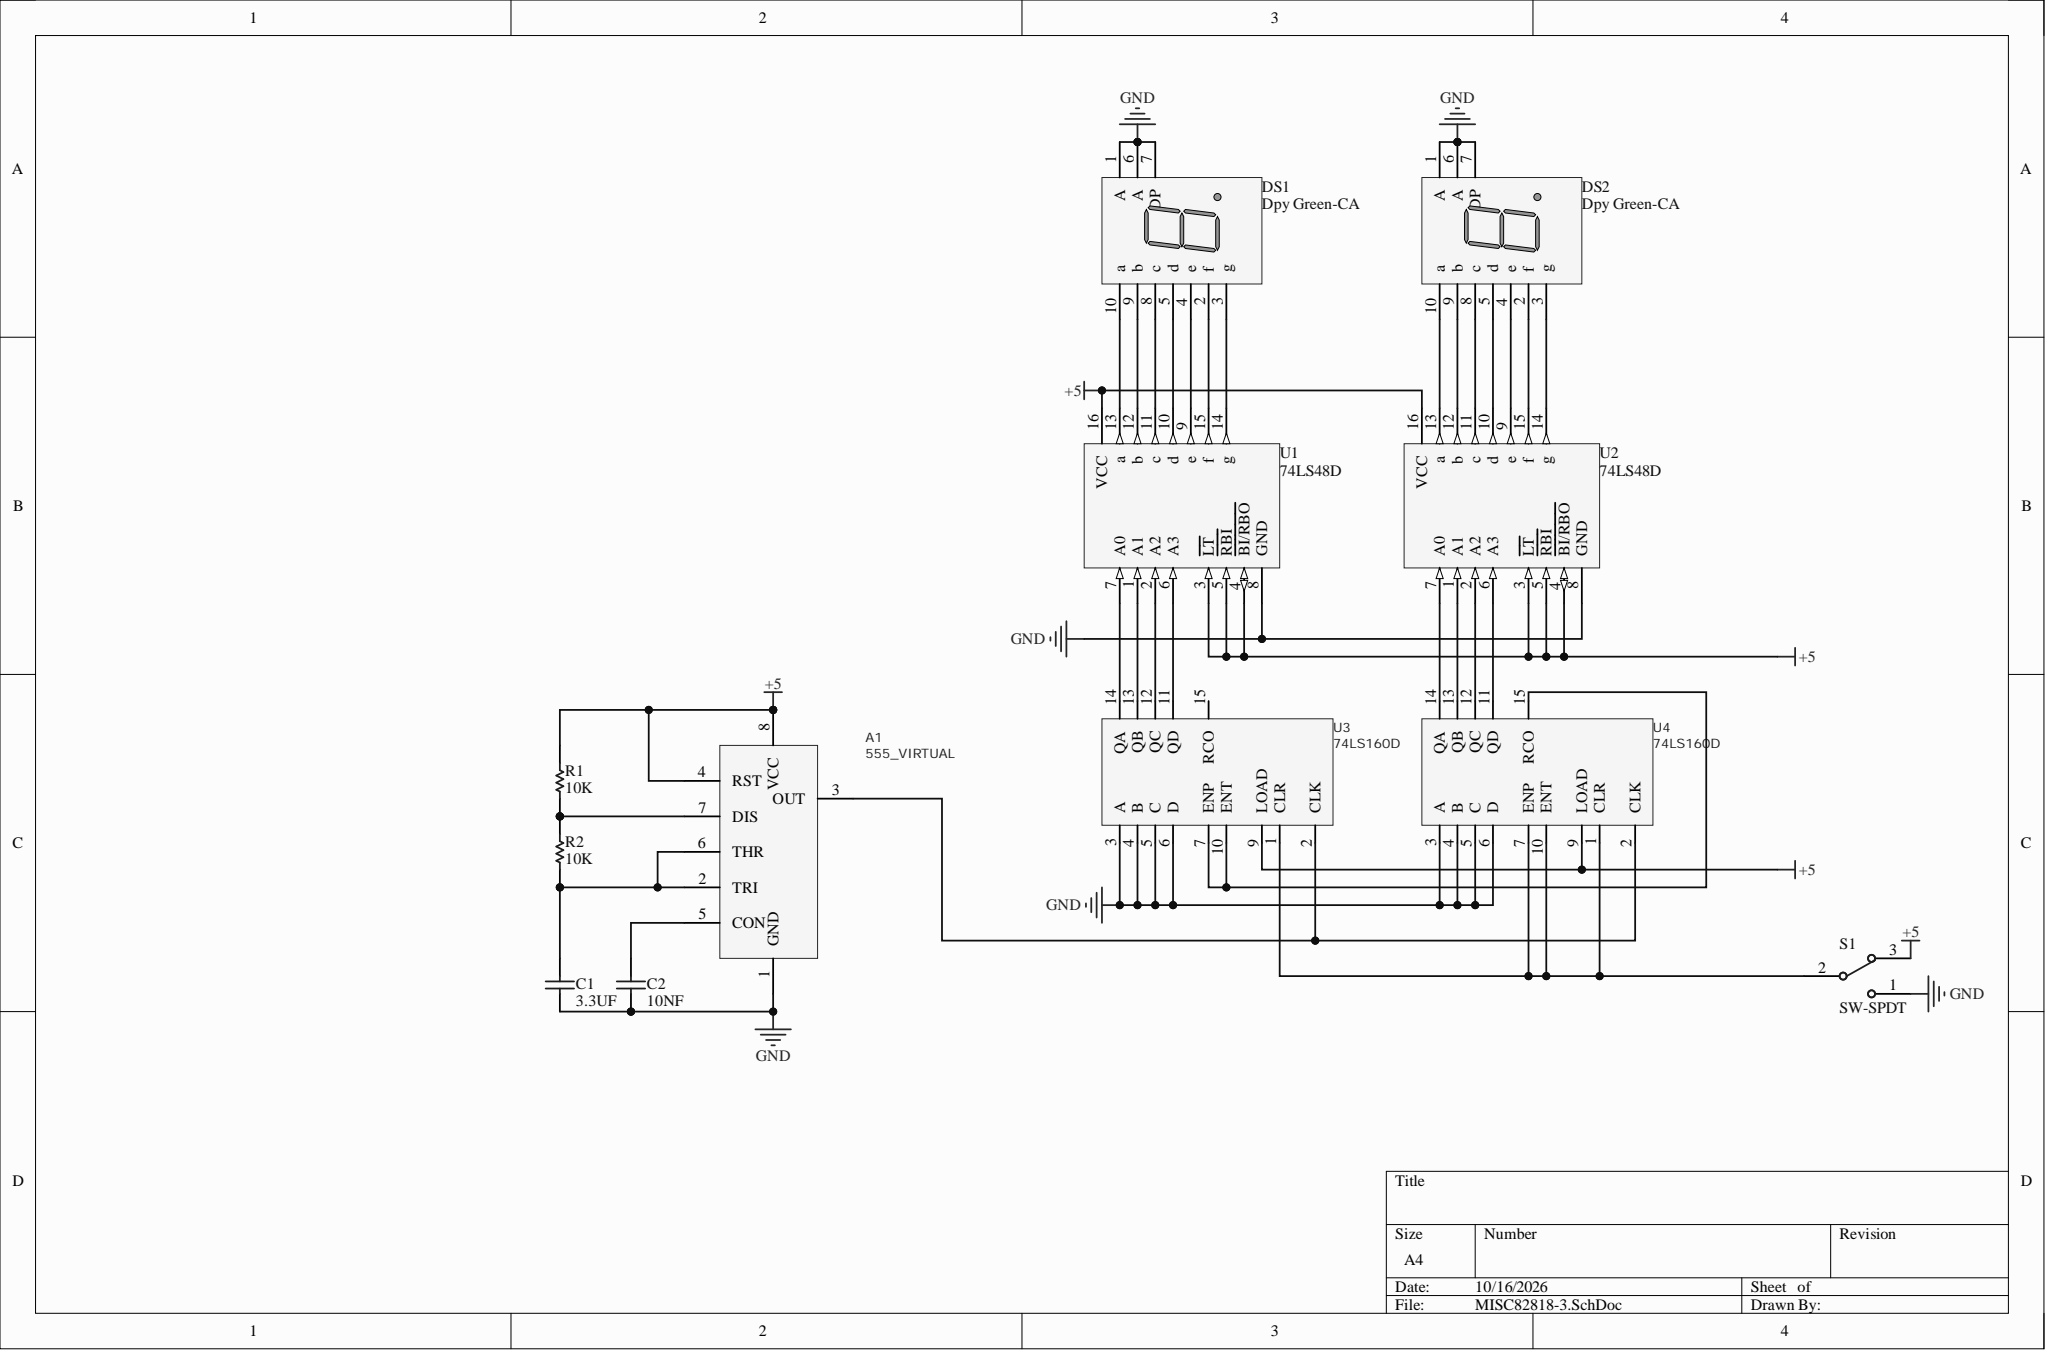Circuit board | Altium Designer | 12 parts | 30 nets
Bill of materials:
Comment,Description,Designator,Footprint,LibRef,Quantity
"555_VIRTUAL","","A1","DIP8","555_VIRTUAL","1"
"3.3UF","Capacitor","C1","RAD-0.3","Cap","1"
"10NF","Capacitor","C2","RAD-0.3","Cap","1"
"Dpy Green-CA","7.62 mm Black Surface Green 7-Segment Display: CA, RH DP","DS1, DS2","A","Dpy Green-CA","2"
"10K","Resistor","R1, R2","AXIAL-0.3","Res1","2"
"SW-SPDT","SPDT Subminiature Toggle Switch, Right Angle Mounting, Vertical Actuation","S1","SW-SPDT-3","SW-SPDT","1"
"74LS48D","BCD-to-Seven-Segment Decoder/Driver","U1, U2","DIP16","SN74LS48D","2"
"74LS160D","","U3, U4","DIP16","74LS160D","2"
Netlist (Protel format):
[
A1
DIP8
555_VIRTUAL



]
[
C1
RAD-0.3
3.3UF



]
[
C2
RAD-0.3
10NF



]
[
DS1
A
Dpy Green-CA



]
[
DS2
A
Dpy Green-CA



]
[
R1
AXIAL-0.3
10K



]
[
R2
AXIAL-0.3
10K



]
[
S1
SW-SPDT-3
SW-SPDT



]
[
U1
DIP16
74LS48D



]
[
U2
DIP16
74LS48D



]
[
U3
DIP16
74LS160D



]
[
U4
DIP16
74LS160D



]
(
NetU3_7
U3-7
U3-10
U4-15
)
(
NetU2_7
U2-7
U4-14
)
(
NetU2_6
U2-6
U4-11
)
(
NetU2_2
U2-2
U4-12
)
(
NetU2_1
U2-1
U4-13
)
(
NetU1_7
U1-7
U3-14
)
(
NetU1_6
U1-6
U3-11
)
(
NetU1_2
U1-2
U3-12
)
(
NetU1_1
U1-1
U3-13
)
(
NetS1_2
S1-2
U3-1
U4-1
U4-7
U4-10
)
(
NetDS2_10
DS2-10
U2-13
)
(
NetDS2_9
DS2-9
U2-12
)
(
NetDS2_8
DS2-8
U2-11
)
(
NetDS2_5
DS2-5
U2-10
)
(
NetDS2_4
DS2-4
U2-9
)
(
NetDS2_3
DS2-3
U2-14
)
(
NetDS2_2
DS2-2
U2-15
)
(
NetDS1_10
DS1-10
U1-13
)
(
NetDS1_9
DS1-9
U1-12
)
(
NetDS1_8
DS1-8
U1-11
)
(
NetDS1_5
DS1-5
U1-10
)
(
NetDS1_4
DS1-4
U1-9
)
(
NetDS1_3
DS1-3
U1-14
)
(
NetDS1_2
DS1-2
U1-15
)
(
NetA1_7
A1-7
R1-1
R2-2
)
(
NetA1_5
A1-5
C2-2
)
(
NetA1_3
A1-3
U3-2
U4-2
)
(
NetA1_2
A1-2
A1-6
C1-2
R2-1
)
(
GND
A1-1
C1-1
C2-1
DS1-1
DS1-6
DS1-7
DS2-1
DS2-6
DS2-7
S1-1
U1-8
U2-8
U3-3
U3-4
U3-5
U3-6
U4-3
U4-4
U4-5
U4-6
)
(
+5
A1-4
A1-8
R1-2
S1-3
U1-3
U1-4
U1-5
U1-16
U2-3
U2-4
U2-5
U2-16
U3-9
U4-9
)